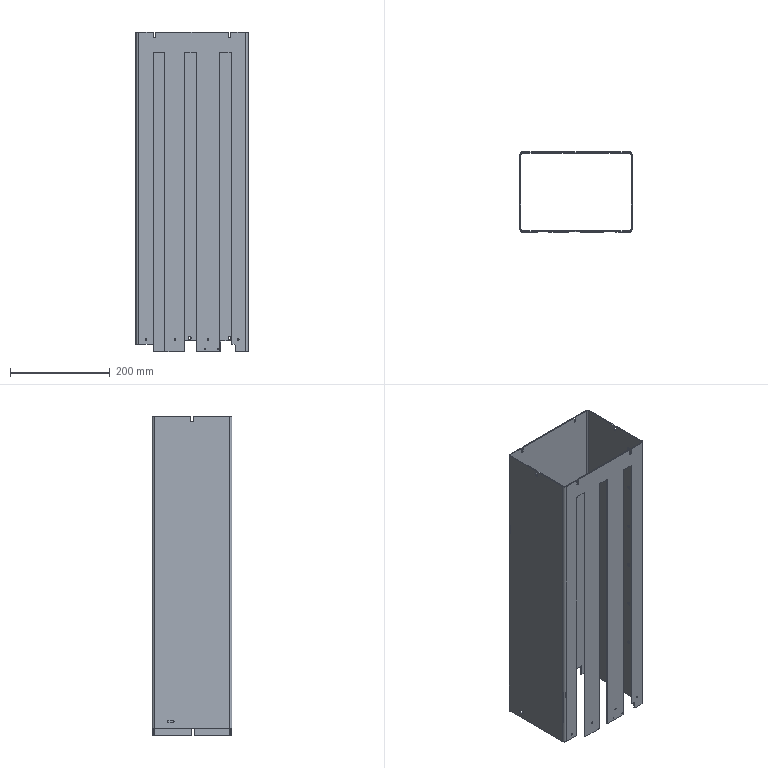Part | NX | features BREP 1 | 1 solid | 122 faces | box 225 x 160 x 642 mm | volume 874897 mm3 | cylinder 67 | plane 55 | commonest cylinder face diameters 6 x20 4 x16 5 x15 3.3 x8 2.5 x4 10 x4